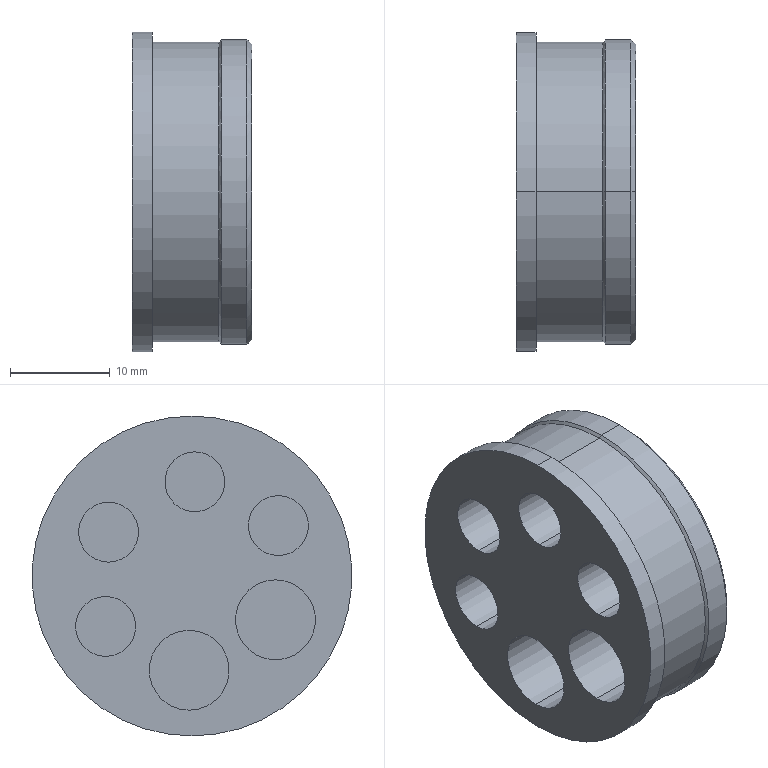Part | SolidWorks | features BaseBody 1 | 1 solid | 34 faces | box 12 x 32 x 32 mm | volume 5499 mm3 | cylinder 20 | plane 10 | cone 4 | commonest cylinder face diameters 6 x8 8 x4 10 x2 30 x2 30.5 x2 32 x2
STEP:
#1=CARTESIAN_POINT('',(-294.521,1906.544,-93.));
#2=VERTEX_POINT('',#1);
#3=CARTESIAN_POINT('',(-294.521,1906.544,-103.));
#4=VERTEX_POINT('',#3);
#5=CARTESIAN_POINT('',(-294.521,1906.544,-98.));
#6=DIRECTION('',(1.,0.,0.));
#7=DIRECTION('',(0.,0.,-1.));
#8=AXIS2_PLACEMENT_3D('',#5,#6,#7);
#9=CIRCLE('',#8,5.);
#10=EDGE_CURVE('',#2,#4,#9,.T.);
#11=ORIENTED_EDGE('',*,*,#10,.F.);
#12=CARTESIAN_POINT('',(-284.521,1906.544,-93.));
#13=VERTEX_POINT('',#12);
#14=CARTESIAN_POINT('',(-289.521,1906.544,-93.));
#15=DIRECTION('',(1.,0.,0.));
#16=VECTOR('',#15,1000.);
#17=LINE('',#14,#16);
#18=EDGE_CURVE('',#2,#13,#17,.T.);
#19=ORIENTED_EDGE('',*,*,#18,.T.);
#20=CARTESIAN_POINT('',(-284.521,1906.544,-103.));
#21=VERTEX_POINT('',#20);
#22=CARTESIAN_POINT('',(-284.521,1906.544,-98.));
#23=DIRECTION('',(-1.,0.,0.));
#24=DIRECTION('',(0.,0.,-1.));
#25=AXIS2_PLACEMENT_3D('',#22,#23,#24);
#26=CIRCLE('',#25,5.);
#27=EDGE_CURVE('',#21,#13,#26,.T.);
#28=ORIENTED_EDGE('',*,*,#27,.F.);
#29=CARTESIAN_POINT('',(-289.521,1906.544,-103.));
#30=DIRECTION('',(1.,0.,0.));
#31=VECTOR('',#30,1000.);
#32=LINE('',#29,#31);
#33=EDGE_CURVE('',#4,#21,#32,.T.);
#34=ORIENTED_EDGE('',*,*,#33,.F.);
#35=EDGE_LOOP('',(#11,#19,#28,#34));
#36=FACE_OUTER_BOUND('',#35,.T.);
#37=CARTESIAN_POINT('',(-289.521,1906.544,-98.));
#38=DIRECTION('',(1.,0.,0.));
#39=DIRECTION('',(0.,0.,-1.));
#40=AXIS2_PLACEMENT_3D('',#37,#38,#39);
#41=CYLINDRICAL_SURFACE('',#40,5.);
#42=ADVANCED_FACE('',(#36),#41,.F.);
#43=CARTESIAN_POINT('',(-284.521,1906.544,-112.75));
#44=VERTEX_POINT('',#43);
#45=CARTESIAN_POINT('',(-284.521,1906.544,-83.25));
#46=VERTEX_POINT('',#45);
#47=CARTESIAN_POINT('',(-284.521,1906.544,-98.));
#48=DIRECTION('',(1.,0.,0.));
#49=DIRECTION('',(0.,0.,1.));
#50=AXIS2_PLACEMENT_3D('',#47,#48,#49);
#51=CIRCLE('',#50,14.75);
#52=EDGE_CURVE('',#44,#46,#51,.T.);
#53=ORIENTED_EDGE('',*,*,#52,.F.);
#54=CARTESIAN_POINT('',(-285.021,1906.544,-113.25));
#55=VERTEX_POINT('',#54);
#56=CARTESIAN_POINT('',(-285.021,1906.544,-113.25));
#57=DIRECTION('',(-0.7071,0.,-0.7071));
#58=VECTOR('',#57,1000.);
#59=LINE('',#56,#58);
#60=EDGE_CURVE('',#44,#55,#59,.T.);
#61=ORIENTED_EDGE('',*,*,#60,.T.);
#62=CARTESIAN_POINT('',(-285.021,1906.544,-82.75));
#63=VERTEX_POINT('',#62);
#64=CARTESIAN_POINT('',(-285.021,1906.544,-98.));
#65=DIRECTION('',(1.,0.,0.));
#66=DIRECTION('',(0.,-0.5043,-0.8635));
#67=AXIS2_PLACEMENT_3D('',#64,#65,#66);
#68=CIRCLE('',#67,15.25);
#69=EDGE_CURVE('',#55,#63,#68,.T.);
#70=ORIENTED_EDGE('',*,*,#69,.T.);
#71=CARTESIAN_POINT('',(-285.021,1906.544,-82.75));
#72=DIRECTION('',(-0.7071,0.,0.7071));
#73=VECTOR('',#72,1000.);
#74=LINE('',#71,#73);
#75=EDGE_CURVE('',#46,#63,#74,.T.);
#76=ORIENTED_EDGE('',*,*,#75,.F.);
#77=EDGE_LOOP('',(#53,#61,#70,#76));
#78=FACE_OUTER_BOUND('',#77,.T.);
#79=CARTESIAN_POINT('',(-285.021,1906.544,-98.));
#80=DIRECTION('',(-1.,0.,0.));
#81=DIRECTION('',(0.,0.,1.));
#82=AXIS2_PLACEMENT_3D('',#79,#80,#81);
#83=CONICAL_SURFACE('',#82,15.25,0.7854);
#84=ADVANCED_FACE('',(#78),#83,.T.);
#85=ORIENTED_EDGE('',*,*,#69,.F.);
#86=CARTESIAN_POINT('',(-287.571,1906.544,-113.25));
#87=VERTEX_POINT('',#86);
#88=CARTESIAN_POINT('',(-284.521,1906.544,-113.25));
#89=DIRECTION('',(-1.,0.,0.));
#90=VECTOR('',#89,1000.);
#91=LINE('',#88,#90);
#92=EDGE_CURVE('',#55,#87,#91,.T.);
#93=ORIENTED_EDGE('',*,*,#92,.T.);
#94=CARTESIAN_POINT('',(-287.571,1906.544,-82.75));
#95=VERTEX_POINT('',#94);
#96=CARTESIAN_POINT('',(-287.571,1906.544,-98.));
#97=DIRECTION('',(1.,0.,0.));
#98=DIRECTION('',(0.,0.,1.));
#99=AXIS2_PLACEMENT_3D('',#96,#97,#98);
#100=CIRCLE('',#99,15.25);
#101=EDGE_CURVE('',#87,#95,#100,.T.);
#102=ORIENTED_EDGE('',*,*,#101,.T.);
#103=CARTESIAN_POINT('',(-284.521,1906.544,-82.75));
#104=DIRECTION('',(-1.,0.,0.));
#105=VECTOR('',#104,1000.);
#106=LINE('',#103,#105);
#107=EDGE_CURVE('',#63,#95,#106,.T.);
#108=ORIENTED_EDGE('',*,*,#107,.F.);
#109=EDGE_LOOP('',(#85,#93,#102,#108));
#110=FACE_OUTER_BOUND('',#109,.T.);
#111=CARTESIAN_POINT('',(-284.521,1906.544,-98.));
#112=DIRECTION('',(-1.,0.,0.));
#113=DIRECTION('',(0.,0.,1.));
#114=AXIS2_PLACEMENT_3D('',#111,#112,#113);
#115=CYLINDRICAL_SURFACE('',#114,15.25);
#116=ADVANCED_FACE('',(#110),#115,.T.);
#117=CARTESIAN_POINT('',(-287.821,1906.544,-113.));
#118=VERTEX_POINT('',#117);
#119=CARTESIAN_POINT('',(-287.821,1906.544,-83.));
#120=VERTEX_POINT('',#119);
#121=CARTESIAN_POINT('',(-287.821,1906.544,-98.));
#122=DIRECTION('',(1.,0.,0.));
#123=DIRECTION('',(0.,0.5043,0.8635));
#124=AXIS2_PLACEMENT_3D('',#121,#122,#123);
#125=CIRCLE('',#124,15.);
#126=EDGE_CURVE('',#118,#120,#125,.T.);
#127=ORIENTED_EDGE('',*,*,#126,.T.);
#128=CARTESIAN_POINT('',(-287.571,1906.544,-82.75));
#129=DIRECTION('',(0.7071,0.,0.7071));
#130=VECTOR('',#129,1000.);
#131=LINE('',#128,#130);
#132=EDGE_CURVE('',#120,#95,#131,.T.);
#133=ORIENTED_EDGE('',*,*,#132,.T.);
#134=ORIENTED_EDGE('',*,*,#101,.F.);
#135=CARTESIAN_POINT('',(-287.571,1906.544,-113.25));
#136=DIRECTION('',(0.7071,0.,-0.7071));
#137=VECTOR('',#136,1000.);
#138=LINE('',#135,#137);
#139=EDGE_CURVE('',#118,#87,#138,.T.);
#140=ORIENTED_EDGE('',*,*,#139,.F.);
#141=EDGE_LOOP('',(#127,#133,#134,#140));
#142=FACE_OUTER_BOUND('',#141,.T.);
#143=CARTESIAN_POINT('',(-287.571,1906.544,-98.));
#144=DIRECTION('',(1.,0.,0.));
#145=DIRECTION('',(0.,0.,-1.));
#146=AXIS2_PLACEMENT_3D('',#143,#144,#145);
#147=CONICAL_SURFACE('',#146,15.25,0.7854);
#148=ADVANCED_FACE('',(#142),#147,.T.);
#149=ORIENTED_EDGE('',*,*,#126,.F.);
#150=CARTESIAN_POINT('',(-294.521,1906.544,-113.));
#151=VERTEX_POINT('',#150);
#152=CARTESIAN_POINT('',(-284.521,1906.544,-113.));
#153=DIRECTION('',(-1.,0.,0.));
#154=VECTOR('',#153,1000.);
#155=LINE('',#152,#154);
#156=EDGE_CURVE('',#118,#151,#155,.T.);
#157=ORIENTED_EDGE('',*,*,#156,.T.);
#158=CARTESIAN_POINT('',(-294.521,1906.544,-83.));
#159=VERTEX_POINT('',#158);
#160=CARTESIAN_POINT('',(-294.521,1906.544,-98.));
#161=DIRECTION('',(1.,0.,0.));
#162=DIRECTION('',(0.,0.,1.));
#163=AXIS2_PLACEMENT_3D('',#160,#161,#162);
#164=CIRCLE('',#163,15.);
#165=EDGE_CURVE('',#151,#159,#164,.T.);
#166=ORIENTED_EDGE('',*,*,#165,.T.);
#167=CARTESIAN_POINT('',(-284.521,1906.544,-83.));
#168=DIRECTION('',(-1.,0.,0.));
#169=VECTOR('',#168,1000.);
#170=LINE('',#167,#169);
#171=EDGE_CURVE('',#120,#159,#170,.T.);
#172=ORIENTED_EDGE('',*,*,#171,.F.);
#173=EDGE_LOOP('',(#149,#157,#166,#172));
#174=FACE_OUTER_BOUND('',#173,.T.);
#175=CARTESIAN_POINT('',(-284.521,1906.544,-98.));
#176=DIRECTION('',(-1.,0.,0.));
#177=DIRECTION('',(0.,0.,1.));
#178=AXIS2_PLACEMENT_3D('',#175,#176,#177);
#179=CYLINDRICAL_SURFACE('',#178,15.);
#180=ADVANCED_FACE('',(#174),#179,.T.);
#181=CARTESIAN_POINT('',(-294.521,1906.544,-114.));
#182=VERTEX_POINT('',#181);
#183=CARTESIAN_POINT('',(-294.521,1906.544,-82.));
#184=VERTEX_POINT('',#183);
#185=CARTESIAN_POINT('',(-294.521,1906.544,-98.));
#186=DIRECTION('',(1.,0.,0.));
#187=DIRECTION('',(0.,0.,1.));
#188=AXIS2_PLACEMENT_3D('',#185,#186,#187);
#189=CIRCLE('',#188,16.);
#190=EDGE_CURVE('',#182,#184,#189,.T.);
#191=ORIENTED_EDGE('',*,*,#190,.F.);
#192=CARTESIAN_POINT('',(-296.521,1906.544,-114.));
#193=VERTEX_POINT('',#192);
#194=CARTESIAN_POINT('',(-294.521,1906.544,-114.));
#195=DIRECTION('',(-1.,0.,0.));
#196=VECTOR('',#195,1000.);
#197=LINE('',#194,#196);
#198=EDGE_CURVE('',#182,#193,#197,.T.);
#199=ORIENTED_EDGE('',*,*,#198,.T.);
#200=CARTESIAN_POINT('',(-296.521,1906.544,-82.));
#201=VERTEX_POINT('',#200);
#202=CARTESIAN_POINT('',(-296.521,1906.544,-98.));
#203=DIRECTION('',(1.,0.,0.));
#204=DIRECTION('',(0.,0.,1.));
#205=AXIS2_PLACEMENT_3D('',#202,#203,#204);
#206=CIRCLE('',#205,16.);
#207=EDGE_CURVE('',#193,#201,#206,.T.);
#208=ORIENTED_EDGE('',*,*,#207,.T.);
#209=CARTESIAN_POINT('',(-294.521,1906.544,-82.));
#210=DIRECTION('',(-1.,0.,0.));
#211=VECTOR('',#210,1000.);
#212=LINE('',#209,#211);
#213=EDGE_CURVE('',#184,#201,#212,.T.);
#214=ORIENTED_EDGE('',*,*,#213,.F.);
#215=EDGE_LOOP('',(#191,#199,#208,#214));
#216=FACE_OUTER_BOUND('',#215,.T.);
#217=CARTESIAN_POINT('',(-294.521,1906.544,-98.));
#218=DIRECTION('',(-1.,0.,0.));
#219=DIRECTION('',(0.,0.,1.));
#220=AXIS2_PLACEMENT_3D('',#217,#218,#219);
#221=CYLINDRICAL_SURFACE('',#220,16.);
#222=ADVANCED_FACE('',(#216),#221,.T.);
#223=CARTESIAN_POINT('',(-285.021,1906.827,-111.43));
#224=VERTEX_POINT('',#223);
#225=CARTESIAN_POINT('',(-285.021,1906.827,-103.43));
#226=VERTEX_POINT('',#225);
#227=CARTESIAN_POINT('',(-285.021,1906.827,-107.43));
#228=DIRECTION('',(-1.,0.,0.));
#229=DIRECTION('',(0.,0.,1.));
#230=AXIS2_PLACEMENT_3D('',#227,#228,#229);
#231=CIRCLE('',#230,4.);
#232=EDGE_CURVE('',#224,#226,#231,.T.);
#233=ORIENTED_EDGE('',*,*,#232,.F.);
#234=CARTESIAN_POINT('',(-296.521,1906.827,-111.43));
#235=VERTEX_POINT('',#234);
#236=CARTESIAN_POINT('',(-290.771,1906.827,-111.43));
#237=DIRECTION('',(-1.,0.,0.));
#238=VECTOR('',#237,1000.);
#239=LINE('',#236,#238);
#240=EDGE_CURVE('',#224,#235,#239,.T.);
#241=ORIENTED_EDGE('',*,*,#240,.T.);
#242=CARTESIAN_POINT('',(-296.521,1906.827,-103.43));
#243=VERTEX_POINT('',#242);
#244=CARTESIAN_POINT('',(-296.521,1906.827,-107.43));
#245=DIRECTION('',(-1.,0.,0.));
#246=DIRECTION('',(0.,0.,1.));
#247=AXIS2_PLACEMENT_3D('',#244,#245,#246);
#248=CIRCLE('',#247,4.);
#249=EDGE_CURVE('',#235,#243,#248,.T.);
#250=ORIENTED_EDGE('',*,*,#249,.T.);
#251=CARTESIAN_POINT('',(-290.771,1906.827,-103.43));
#252=DIRECTION('',(-1.,0.,0.));
#253=VECTOR('',#252,1000.);
#254=LINE('',#251,#253);
#255=EDGE_CURVE('',#226,#243,#254,.T.);
#256=ORIENTED_EDGE('',*,*,#255,.F.);
#257=EDGE_LOOP('',(#233,#241,#250,#256));
#258=FACE_OUTER_BOUND('',#257,.T.);
#259=CARTESIAN_POINT('',(-290.771,1906.827,-107.43));
#260=DIRECTION('',(-1.,0.,0.));
#261=DIRECTION('',(0.,0.,1.));
#262=AXIS2_PLACEMENT_3D('',#259,#260,#261);
#263=CYLINDRICAL_SURFACE('',#262,4.);
#264=ADVANCED_FACE('',(#258),#263,.F.);
#265=CARTESIAN_POINT('',(-285.021,1906.261,-91.57));
#266=VERTEX_POINT('',#265);
#267=CARTESIAN_POINT('',(-285.021,1906.261,-85.57));
#268=VERTEX_POINT('',#267);
#269=CARTESIAN_POINT('',(-285.021,1906.261,-88.57));
#270=DIRECTION('',(-1.,0.,0.));
#271=DIRECTION('',(0.,0.,1.));
#272=AXIS2_PLACEMENT_3D('',#269,#270,#271);
#273=CIRCLE('',#272,3.);
#274=EDGE_CURVE('',#266,#268,#273,.T.);
#275=ORIENTED_EDGE('',*,*,#274,.F.);
#276=CARTESIAN_POINT('',(-296.521,1906.261,-91.57));
#277=VERTEX_POINT('',#276);
#278=CARTESIAN_POINT('',(-290.771,1906.261,-91.57));
#279=DIRECTION('',(-1.,0.,0.));
#280=VECTOR('',#279,1000.);
#281=LINE('',#278,#280);
#282=EDGE_CURVE('',#266,#277,#281,.T.);
#283=ORIENTED_EDGE('',*,*,#282,.T.);
#284=CARTESIAN_POINT('',(-296.521,1906.261,-85.57));
#285=VERTEX_POINT('',#284);
#286=CARTESIAN_POINT('',(-296.521,1906.261,-88.57));
#287=DIRECTION('',(-1.,0.,0.));
#288=DIRECTION('',(0.,0.,1.));
#289=AXIS2_PLACEMENT_3D('',#286,#287,#288);
#290=CIRCLE('',#289,3.);
#291=EDGE_CURVE('',#277,#285,#290,.T.);
#292=ORIENTED_EDGE('',*,*,#291,.T.);
#293=CARTESIAN_POINT('',(-290.771,1906.261,-85.57));
#294=DIRECTION('',(-1.,0.,0.));
#295=VECTOR('',#294,1000.);
#296=LINE('',#293,#295);
#297=EDGE_CURVE('',#268,#285,#296,.T.);
#298=ORIENTED_EDGE('',*,*,#297,.F.);
#299=EDGE_LOOP('',(#275,#283,#292,#298));
#300=FACE_OUTER_BOUND('',#299,.T.);
#301=CARTESIAN_POINT('',(-290.771,1906.261,-88.57));
#302=DIRECTION('',(-1.,0.,0.));
#303=DIRECTION('',(0.,0.,1.));
#304=AXIS2_PLACEMENT_3D('',#301,#302,#303);
#305=CYLINDRICAL_SURFACE('',#304,3.);
#306=ADVANCED_FACE('',(#300),#305,.F.);
#307=CARTESIAN_POINT('',(-285.021,1915.179,-106.043));
#308=VERTEX_POINT('',#307);
#309=CARTESIAN_POINT('',(-285.021,1915.179,-100.043));
#310=VERTEX_POINT('',#309);
#311=CARTESIAN_POINT('',(-285.021,1915.179,-103.043));
#312=DIRECTION('',(-1.,0.,0.));
#313=DIRECTION('',(0.,0.,1.));
#314=AXIS2_PLACEMENT_3D('',#311,#312,#313);
#315=CIRCLE('',#314,3.);
#316=EDGE_CURVE('',#308,#310,#315,.T.);
#317=ORIENTED_EDGE('',*,*,#316,.F.);
#318=CARTESIAN_POINT('',(-296.521,1915.179,-106.043));
#319=VERTEX_POINT('',#318);
#320=CARTESIAN_POINT('',(-290.771,1915.179,-106.043));
#321=DIRECTION('',(-1.,0.,0.));
#322=VECTOR('',#321,1000.);
#323=LINE('',#320,#322);
#324=EDGE_CURVE('',#308,#319,#323,.T.);
#325=ORIENTED_EDGE('',*,*,#324,.T.);
#326=CARTESIAN_POINT('',(-296.521,1915.179,-100.043));
#327=VERTEX_POINT('',#326);
#328=CARTESIAN_POINT('',(-296.521,1915.179,-103.043));
#329=DIRECTION('',(-1.,0.,0.));
#330=DIRECTION('',(0.,0.,1.));
#331=AXIS2_PLACEMENT_3D('',#328,#329,#330);
#332=CIRCLE('',#331,3.);
#333=EDGE_CURVE('',#319,#327,#332,.T.);
#334=ORIENTED_EDGE('',*,*,#333,.T.);
#335=CARTESIAN_POINT('',(-290.771,1915.179,-100.043));
#336=DIRECTION('',(-1.,0.,0.));
#337=VECTOR('',#336,1000.);
#338=LINE('',#335,#337);
#339=EDGE_CURVE('',#310,#327,#338,.T.);
#340=ORIENTED_EDGE('',*,*,#339,.F.);
#341=EDGE_LOOP('',(#317,#325,#334,#340));
#342=FACE_OUTER_BOUND('',#341,.T.);
#343=CARTESIAN_POINT('',(-290.771,1915.179,-103.043));
#344=DIRECTION('',(-1.,0.,0.));
#345=DIRECTION('',(0.,0.,1.));
#346=AXIS2_PLACEMENT_3D('',#343,#344,#345);
#347=CYLINDRICAL_SURFACE('',#346,3.);
#348=ADVANCED_FACE('',(#342),#347,.F.);
#349=CARTESIAN_POINT('',(-285.021,1897.909,-95.957));
#350=VERTEX_POINT('',#349);
#351=CARTESIAN_POINT('',(-285.021,1897.909,-89.957));
#352=VERTEX_POINT('',#351);
#353=CARTESIAN_POINT('',(-285.021,1897.909,-92.957));
#354=DIRECTION('',(-1.,0.,0.));
#355=DIRECTION('',(0.,0.,1.));
#356=AXIS2_PLACEMENT_3D('',#353,#354,#355);
#357=CIRCLE('',#356,3.);
#358=EDGE_CURVE('',#350,#352,#357,.T.);
#359=ORIENTED_EDGE('',*,*,#358,.F.);
#360=CARTESIAN_POINT('',(-296.521,1897.909,-95.957));
#361=VERTEX_POINT('',#360);
#362=CARTESIAN_POINT('',(-290.771,1897.909,-95.957));
#363=DIRECTION('',(-1.,0.,0.));
#364=VECTOR('',#363,1000.);
#365=LINE('',#362,#364);
#366=EDGE_CURVE('',#350,#361,#365,.T.);
#367=ORIENTED_EDGE('',*,*,#366,.T.);
#368=CARTESIAN_POINT('',(-296.521,1897.909,-89.957));
#369=VERTEX_POINT('',#368);
#370=CARTESIAN_POINT('',(-296.521,1897.909,-92.957));
#371=DIRECTION('',(-1.,0.,0.));
#372=DIRECTION('',(0.,0.,1.));
#373=AXIS2_PLACEMENT_3D('',#370,#371,#372);
#374=CIRCLE('',#373,3.);
#375=EDGE_CURVE('',#361,#369,#374,.T.);
#376=ORIENTED_EDGE('',*,*,#375,.T.);
#377=CARTESIAN_POINT('',(-290.771,1897.909,-89.957));
#378=DIRECTION('',(-1.,0.,0.));
#379=VECTOR('',#378,1000.);
#380=LINE('',#377,#379);
#381=EDGE_CURVE('',#352,#369,#380,.T.);
#382=ORIENTED_EDGE('',*,*,#381,.F.);
#383=EDGE_LOOP('',(#359,#367,#376,#382));
#384=FACE_OUTER_BOUND('',#383,.T.);
#385=CARTESIAN_POINT('',(-290.771,1897.909,-92.957));
#386=DIRECTION('',(-1.,0.,0.));
#387=DIRECTION('',(0.,0.,1.));
#388=AXIS2_PLACEMENT_3D('',#385,#386,#387);
#389=CYLINDRICAL_SURFACE('',#388,3.);
#390=ADVANCED_FACE('',(#384),#389,.F.);
#391=CARTESIAN_POINT('',(-285.021,1914.896,-96.613));
#392=VERTEX_POINT('',#391);
#393=CARTESIAN_POINT('',(-285.021,1914.896,-90.613));
#394=VERTEX_POINT('',#393);
#395=CARTESIAN_POINT('',(-285.021,1914.896,-93.613));
#396=DIRECTION('',(-1.,0.,0.));
#397=DIRECTION('',(0.,0.,1.));
#398=AXIS2_PLACEMENT_3D('',#395,#396,#397);
#399=CIRCLE('',#398,3.);
#400=EDGE_CURVE('',#392,#394,#399,.T.);
#401=ORIENTED_EDGE('',*,*,#400,.F.);
#402=CARTESIAN_POINT('',(-296.521,1914.896,-96.613));
#403=VERTEX_POINT('',#402);
#404=CARTESIAN_POINT('',(-290.771,1914.896,-96.613));
#405=DIRECTION('',(-1.,0.,0.));
#406=VECTOR('',#405,1000.);
#407=LINE('',#404,#406);
#408=EDGE_CURVE('',#392,#403,#407,.T.);
#409=ORIENTED_EDGE('',*,*,#408,.T.);
#410=CARTESIAN_POINT('',(-296.521,1914.896,-90.613));
#411=VERTEX_POINT('',#410);
#412=CARTESIAN_POINT('',(-296.521,1914.896,-93.613));
#413=DIRECTION('',(-1.,0.,0.));
#414=DIRECTION('',(0.,0.,1.));
#415=AXIS2_PLACEMENT_3D('',#412,#413,#414);
#416=CIRCLE('',#415,3.);
#417=EDGE_CURVE('',#403,#411,#416,.T.);
#418=ORIENTED_EDGE('',*,*,#417,.T.);
#419=CARTESIAN_POINT('',(-290.771,1914.896,-90.613));
#420=DIRECTION('',(-1.,0.,0.));
#421=VECTOR('',#420,1000.);
#422=LINE('',#419,#421);
#423=EDGE_CURVE('',#394,#411,#422,.T.);
#424=ORIENTED_EDGE('',*,*,#423,.F.);
#425=EDGE_LOOP('',(#401,#409,#418,#424));
#426=FACE_OUTER_BOUND('',#425,.T.);
#427=CARTESIAN_POINT('',(-290.771,1914.896,-93.613));
#428=DIRECTION('',(-1.,0.,0.));
#429=DIRECTION('',(0.,0.,1.));
#430=AXIS2_PLACEMENT_3D('',#427,#428,#429);
#431=CYLINDRICAL_SURFACE('',#430,3.);
#432=ADVANCED_FACE('',(#426),#431,.F.);
#433=CARTESIAN_POINT('',(-285.021,1898.192,-106.387));
#434=VERTEX_POINT('',#433);
#435=CARTESIAN_POINT('',(-285.021,1898.192,-98.387));
#436=VERTEX_POINT('',#435);
#437=CARTESIAN_POINT('',(-285.021,1898.192,-102.387));
#438=DIRECTION('',(-1.,0.,0.));
#439=DIRECTION('',(0.,0.,1.));
#440=AXIS2_PLACEMENT_3D('',#437,#438,#439);
#441=CIRCLE('',#440,4.);
#442=EDGE_CURVE('',#434,#436,#441,.T.);
#443=ORIENTED_EDGE('',*,*,#442,.F.);
#444=CARTESIAN_POINT('',(-296.521,1898.192,-106.387));
#445=VERTEX_POINT('',#444);
#446=CARTESIAN_POINT('',(-290.771,1898.192,-106.387));
#447=DIRECTION('',(-1.,0.,0.));
#448=VECTOR('',#447,1000.);
#449=LINE('',#446,#448);
#450=EDGE_CURVE('',#434,#445,#449,.T.);
#451=ORIENTED_EDGE('',*,*,#450,.T.);
#452=CARTESIAN_POINT('',(-296.521,1898.192,-98.387));
#453=VERTEX_POINT('',#452);
#454=CARTESIAN_POINT('',(-296.521,1898.192,-102.387));
#455=DIRECTION('',(-1.,0.,0.));
#456=DIRECTION('',(0.,0.,1.));
#457=AXIS2_PLACEMENT_3D('',#454,#455,#456);
#458=CIRCLE('',#457,4.);
#459=EDGE_CURVE('',#445,#453,#458,.T.);
#460=ORIENTED_EDGE('',*,*,#459,.T.);
#461=CARTESIAN_POINT('',(-290.771,1898.192,-98.387));
#462=DIRECTION('',(-1.,0.,0.));
#463=VECTOR('',#462,1000.);
#464=LINE('',#461,#463);
#465=EDGE_CURVE('',#436,#453,#464,.T.);
#466=ORIENTED_EDGE('',*,*,#465,.F.);
#467=EDGE_LOOP('',(#443,#451,#460,#466));
#468=FACE_OUTER_BOUND('',#467,.T.);
#469=CARTESIAN_POINT('',(-290.771,1898.192,-102.387));
#470=DIRECTION('',(-1.,0.,0.));
#471=DIRECTION('',(0.,0.,1.));
#472=AXIS2_PLACEMENT_3D('',#469,#470,#471);
#473=CYLINDRICAL_SURFACE('',#472,4.);
#474=ADVANCED_FACE('',(#468),#473,.F.);
#475=ORIENTED_EDGE('',*,*,#27,.T.);
#476=CARTESIAN_POINT('',(-284.521,1906.544,-98.));
#477=DIRECTION('',(-1.,0.,0.));
#478=DIRECTION('',(0.,0.,-1.));
#479=AXIS2_PLACEMENT_3D('',#476,#477,#478);
#480=CIRCLE('',#479,5.);
#481=EDGE_CURVE('',#13,#21,#480,.T.);
#482=ORIENTED_EDGE('',*,*,#481,.T.);
#483=EDGE_LOOP('',(#475,#482));
#484=FACE_BOUND('',#483,.T.);
#485=CARTESIAN_POINT('',(-284.521,1906.544,-98.));
#486=DIRECTION('',(1.,0.,0.));
#487=DIRECTION('',(0.,0.,1.));
#488=AXIS2_PLACEMENT_3D('',#485,#486,#487);
#489=CIRCLE('',#488,14.75);
#490=EDGE_CURVE('',#46,#44,#489,.T.);
#491=ORIENTED_EDGE('',*,*,#490,.T.);
#492=ORIENTED_EDGE('',*,*,#52,.T.);
#493=EDGE_LOOP('',(#491,#492));
#494=FACE_OUTER_BOUND('',#493,.T.);
#495=CARTESIAN_POINT('',(-284.521,1906.544,-98.));
#496=DIRECTION('',(1.,0.,0.));
#497=DIRECTION('',(0.,0.,-1.));
#498=AXIS2_PLACEMENT_3D('',#495,#496,#497);
#499=PLANE('',#498);
#500=ADVANCED_FACE('',(#484,#494),#499,.T.);
#501=ORIENTED_EDGE('',*,*,#18,.F.);
#502=CARTESIAN_POINT('',(-294.521,1906.544,-98.));
#503=DIRECTION('',(1.,0.,0.));
#504=DIRECTION('',(0.,0.,-1.));
#505=AXIS2_PLACEMENT_3D('',#502,#503,#504);
#506=CIRCLE('',#505,5.);
#507=EDGE_CURVE('',#4,#2,#506,.T.);
#508=ORIENTED_EDGE('',*,*,#507,.F.);
#509=ORIENTED_EDGE('',*,*,#33,.T.);
#510=ORIENTED_EDGE('',*,*,#481,.F.);
#511=EDGE_LOOP('',(#501,#508,#509,#510));
#512=FACE_OUTER_BOUND('',#511,.T.);
#513=CARTESIAN_POINT('',(-289.521,1906.544,-98.));
#514=DIRECTION('',(1.,0.,0.));
#515=DIRECTION('',(0.,0.,-1.));
#516=AXIS2_PLACEMENT_3D('',#513,#514,#515);
#517=CYLINDRICAL_SURFACE('',#516,5.);
#518=ADVANCED_FACE('',(#512),#517,.F.);
#519=ORIENTED_EDGE('',*,*,#60,.F.);
#520=ORIENTED_EDGE('',*,*,#490,.F.);
#521=ORIENTED_EDGE('',*,*,#75,.T.);
#522=CARTESIAN_POINT('',(-285.021,1906.544,-98.));
#523=DIRECTION('',(1.,0.,0.));
#524=DIRECTION('',(0.,-0.5043,-0.8635));
#525=AXIS2_PLACEMENT_3D('',#522,#523,#524);
#526=CIRCLE('',#525,15.25);
#527=EDGE_CURVE('',#63,#55,#526,.T.);
#528=ORIENTED_EDGE('',*,*,#527,.T.);
#529=EDGE_LOOP('',(#519,#520,#521,#528));
#530=FACE_OUTER_BOUND('',#529,.T.);
#531=CARTESIAN_POINT('',(-285.021,1906.544,-98.));
#532=DIRECTION('',(-1.,0.,0.));
#533=DIRECTION('',(0.,0.,1.));
#534=AXIS2_PLACEMENT_3D('',#531,#532,#533);
#535=CONICAL_SURFACE('',#534,15.25,0.7854);
#536=ADVANCED_FACE('',(#530),#535,.T.);
#537=ORIENTED_EDGE('',*,*,#507,.T.);
#538=ORIENTED_EDGE('',*,*,#10,.T.);
#539=EDGE_LOOP('',(#537,#538));
#540=FACE_OUTER_BOUND('',#539,.T.);
#541=CARTESIAN_POINT('',(-294.521,1906.544,-98.));
#542=DIRECTION('',(1.,0.,0.));
#543=DIRECTION('',(0.,0.,-1.));
#544=AXIS2_PLACEMENT_3D('',#541,#542,#543);
#545=PLANE('',#544);
#546=ADVANCED_FACE('',(#540),#545,.T.);
#547=ORIENTED_EDGE('',*,*,#92,.F.);
#548=ORIENTED_EDGE('',*,*,#527,.F.);
#549=ORIENTED_EDGE('',*,*,#107,.T.);
#550=CARTESIAN_POINT('',(-287.571,1906.544,-98.));
#551=DIRECTION('',(1.,0.,0.));
#552=DIRECTION('',(0.,0.,1.));
#553=AXIS2_PLACEMENT_3D('',#550,#551,#552);
#554=CIRCLE('',#553,15.25);
#555=EDGE_CURVE('',#95,#87,#554,.T.);
#556=ORIENTED_EDGE('',*,*,#555,.T.);
#557=EDGE_LOOP('',(#547,#548,#549,#556));
#558=FACE_OUTER_BOUND('',#557,.T.);
#559=CARTESIAN_POINT('',(-284.521,1906.544,-98.));
#560=DIRECTION('',(-1.,0.,0.));
#561=DIRECTION('',(0.,0.,1.));
#562=AXIS2_PLACEMENT_3D('',#559,#560,#561);
#563=CYLINDRICAL_SURFACE('',#562,15.25);
#564=ADVANCED_FACE('',(#558),#563,.T.);
#565=ORIENTED_EDGE('',*,*,#132,.F.);
#566=CARTESIAN_POINT('',(-287.821,1906.544,-98.));
#567=DIRECTION('',(1.,0.,0.));
#568=DIRECTION('',(0.,0.5043,0.8635));
#569=AXIS2_PLACEMENT_3D('',#566,#567,#568);
#570=CIRCLE('',#569,15.);
#571=EDGE_CURVE('',#120,#118,#570,.T.);
#572=ORIENTED_EDGE('',*,*,#571,.T.);
#573=ORIENTED_EDGE('',*,*,#139,.T.);
#574=ORIENTED_EDGE('',*,*,#555,.F.);
#575=EDGE_LOOP('',(#565,#572,#573,#574));
#576=FACE_OUTER_BOUND('',#575,.T.);
#577=CARTESIAN_POINT('',(-287.571,1906.544,-98.));
#578=DIRECTION('',(1.,0.,0.));
#579=DIRECTION('',(0.,0.,-1.));
#580=AXIS2_PLACEMENT_3D('',#577,#578,#579);
#581=CONICAL_SURFACE('',#580,15.25,0.7854);
#582=ADVANCED_FACE('',(#576),#581,.T.);
#583=ORIENTED_EDGE('',*,*,#156,.F.);
#584=ORIENTED_EDGE('',*,*,#571,.F.);
#585=ORIENTED_EDGE('',*,*,#171,.T.);
#586=CARTESIAN_POINT('',(-294.521,1906.544,-98.));
#587=DIRECTION('',(1.,0.,0.));
#588=DIRECTION('',(0.,0.,1.));
#589=AXIS2_PLACEMENT_3D('',#586,#587,#588);
#590=CIRCLE('',#589,15.);
#591=EDGE_CURVE('',#159,#151,#590,.T.);
#592=ORIENTED_EDGE('',*,*,#591,.T.);
#593=EDGE_LOOP('',(#583,#584,#585,#592));
#594=FACE_OUTER_BOUND('',#593,.T.);
#595=CARTESIAN_POINT('',(-284.521,1906.544,-98.));
#596=DIRECTION('',(-1.,0.,0.));
#597=DIRECTION('',(0.,0.,1.));
#598=AXIS2_PLACEMENT_3D('',#595,#596,#597);
#599=CYLINDRICAL_SURFACE('',#598,15.);
#600=ADVANCED_FACE('',(#594),#599,.T.);
#601=ORIENTED_EDGE('',*,*,#591,.F.);
#602=ORIENTED_EDGE('',*,*,#165,.F.);
#603=EDGE_LOOP('',(#601,#602));
#604=FACE_BOUND('',#603,.T.);
#605=CARTESIAN_POINT('',(-294.521,1906.544,-98.));
#606=DIRECTION('',(1.,0.,0.));
#607=DIRECTION('',(0.,0.,1.));
#608=AXIS2_PLACEMENT_3D('',#605,#606,#607);
#609=CIRCLE('',#608,16.);
#610=EDGE_CURVE('',#184,#182,#609,.T.);
#611=ORIENTED_EDGE('',*,*,#610,.T.);
#612=ORIENTED_EDGE('',*,*,#190,.T.);
#613=EDGE_LOOP('',(#611,#612));
#614=FACE_OUTER_BOUND('',#613,.T.);
#615=CARTESIAN_POINT('',(-294.521,1906.544,-98.));
#616=DIRECTION('',(1.,0.,0.));
#617=DIRECTION('',(0.,0.,-1.));
#618=AXIS2_PLACEMENT_3D('',#615,#616,#617);
#619=PLANE('',#618);
#620=ADVANCED_FACE('',(#604,#614),#619,.T.);
#621=ORIENTED_EDGE('',*,*,#198,.F.);
#622=ORIENTED_EDGE('',*,*,#610,.F.);
#623=ORIENTED_EDGE('',*,*,#213,.T.);
#624=CARTESIAN_POINT('',(-296.521,1906.544,-98.));
#625=DIRECTION('',(1.,0.,0.));
#626=DIRECTION('',(0.,0.,1.));
#627=AXIS2_PLACEMENT_3D('',#624,#625,#626);
#628=CIRCLE('',#627,16.);
#629=EDGE_CURVE('',#201,#193,#628,.T.);
#630=ORIENTED_EDGE('',*,*,#629,.T.);
#631=EDGE_LOOP('',(#621,#622,#623,#630));
#632=FACE_OUTER_BOUND('',#631,.T.);
#633=CARTESIAN_POINT('',(-294.521,1906.544,-98.));
#634=DIRECTION('',(-1.,0.,0.));
#635=DIRECTION('',(0.,0.,1.));
#636=AXIS2_PLACEMENT_3D('',#633,#634,#635);
#637=CYLINDRICAL_SURFACE('',#636,16.);
#638=ADVANCED_FACE('',(#632),#637,.T.);
#639=CARTESIAN_POINT('',(-296.521,1906.827,-107.43));
#640=DIRECTION('',(-1.,0.,0.));
#641=DIRECTION('',(0.,0.,1.));
#642=AXIS2_PLACEMENT_3D('',#639,#640,#641);
#643=CIRCLE('',#642,4.);
#644=EDGE_CURVE('',#243,#235,#643,.T.);
#645=ORIENTED_EDGE('',*,*,#644,.F.);
#646=ORIENTED_EDGE('',*,*,#249,.F.);
#647=EDGE_LOOP('',(#645,#646));
#648=FACE_BOUND('',#647,.T.);
#649=CARTESIAN_POINT('',(-296.521,1906.261,-88.57));
#650=DIRECTION('',(-1.,0.,0.));
#651=DIRECTION('',(0.,0.,1.));
#652=AXIS2_PLACEMENT_3D('',#649,#650,#651);
#653=CIRCLE('',#652,3.);
#654=EDGE_CURVE('',#285,#277,#653,.T.);
#655=ORIENTED_EDGE('',*,*,#654,.F.);
#656=ORIENTED_EDGE('',*,*,#291,.F.);
#657=EDGE_LOOP('',(#655,#656));
#658=FACE_BOUND('',#657,.T.);
#659=CARTESIAN_POINT('',(-296.521,1915.179,-103.043));
#660=DIRECTION('',(-1.,0.,0.));
#661=DIRECTION('',(0.,0.,1.));
#662=AXIS2_PLACEMENT_3D('',#659,#660,#661);
#663=CIRCLE('',#662,3.);
#664=EDGE_CURVE('',#327,#319,#663,.T.);
#665=ORIENTED_EDGE('',*,*,#664,.F.);
#666=ORIENTED_EDGE('',*,*,#333,.F.);
#667=EDGE_LOOP('',(#665,#666));
#668=FACE_BOUND('',#667,.T.);
#669=CARTESIAN_POINT('',(-296.521,1897.909,-92.957));
#670=DIRECTION('',(-1.,0.,0.));
#671=DIRECTION('',(0.,0.,1.));
#672=AXIS2_PLACEMENT_3D('',#669,#670,#671);
#673=CIRCLE('',#672,3.);
#674=EDGE_CURVE('',#369,#361,#673,.T.);
#675=ORIENTED_EDGE('',*,*,#674,.F.);
#676=ORIENTED_EDGE('',*,*,#375,.F.);
#677=EDGE_LOOP('',(#675,#676));
#678=FACE_BOUND('',#677,.T.);
#679=CARTESIAN_POINT('',(-296.521,1914.896,-93.613));
#680=DIRECTION('',(-1.,0.,0.));
#681=DIRECTION('',(0.,0.,1.));
#682=AXIS2_PLACEMENT_3D('',#679,#680,#681);
#683=CIRCLE('',#682,3.);
#684=EDGE_CURVE('',#411,#403,#683,.T.);
#685=ORIENTED_EDGE('',*,*,#684,.F.);
#686=ORIENTED_EDGE('',*,*,#417,.F.);
#687=EDGE_LOOP('',(#685,#686));
#688=FACE_BOUND('',#687,.T.);
#689=CARTESIAN_POINT('',(-296.521,1898.192,-102.387));
#690=DIRECTION('',(-1.,0.,0.));
#691=DIRECTION('',(0.,0.,1.));
#692=AXIS2_PLACEMENT_3D('',#689,#690,#691);
#693=CIRCLE('',#692,4.);
#694=EDGE_CURVE('',#453,#445,#693,.T.);
#695=ORIENTED_EDGE('',*,*,#694,.F.);
#696=ORIENTED_EDGE('',*,*,#459,.F.);
#697=EDGE_LOOP('',(#695,#696));
#698=FACE_BOUND('',#697,.T.);
#699=ORIENTED_EDGE('',*,*,#629,.F.);
#700=ORIENTED_EDGE('',*,*,#207,.F.);
#701=EDGE_LOOP('',(#699,#700));
#702=FACE_OUTER_BOUND('',#701,.T.);
#703=CARTESIAN_POINT('',(-296.521,1906.544,-98.));
#704=DIRECTION('',(1.,0.,0.));
#705=DIRECTION('',(0.,0.,-1.));
#706=AXIS2_PLACEMENT_3D('',#703,#704,#705);
#707=PLANE('',#706);
#708=ADVANCED_FACE('',(#648,#658,#668,#678,#688,#698,#702),#707,.F.);
#709=ORIENTED_EDGE('',*,*,#240,.F.);
#710=CARTESIAN_POINT('',(-285.021,1906.827,-107.43));
#711=DIRECTION('',(-1.,0.,0.));
#712=DIRECTION('',(0.,0.,1.));
#713=AXIS2_PLACEMENT_3D('',#710,#711,#712);
#714=CIRCLE('',#713,4.);
#715=EDGE_CURVE('',#226,#224,#714,.T.);
#716=ORIENTED_EDGE('',*,*,#715,.F.);
#717=ORIENTED_EDGE('',*,*,#255,.T.);
#718=ORIENTED_EDGE('',*,*,#644,.T.);
#719=EDGE_LOOP('',(#709,#716,#717,#718));
#720=FACE_OUTER_BOUND('',#719,.T.);
#721=CARTESIAN_POINT('',(-290.771,1906.827,-107.43));
#722=DIRECTION('',(-1.,0.,0.));
#723=DIRECTION('',(0.,0.,1.));
#724=AXIS2_PLACEMENT_3D('',#721,#722,#723);
#725=CYLINDRICAL_SURFACE('',#724,4.);
#726=ADVANCED_FACE('',(#720),#725,.F.);
#727=ORIENTED_EDGE('',*,*,#282,.F.);
#728=CARTESIAN_POINT('',(-285.021,1906.261,-88.57));
#729=DIRECTION('',(-1.,0.,0.));
#730=DIRECTION('',(0.,0.,1.));
#731=AXIS2_PLACEMENT_3D('',#728,#729,#730);
#732=CIRCLE('',#731,3.);
#733=EDGE_CURVE('',#268,#266,#732,.T.);
#734=ORIENTED_EDGE('',*,*,#733,.F.);
#735=ORIENTED_EDGE('',*,*,#297,.T.);
#736=ORIENTED_EDGE('',*,*,#654,.T.);
#737=EDGE_LOOP('',(#727,#734,#735,#736));
#738=FACE_OUTER_BOUND('',#737,.T.);
#739=CARTESIAN_POINT('',(-290.771,1906.261,-88.57));
#740=DIRECTION('',(-1.,0.,0.));
#741=DIRECTION('',(0.,0.,1.));
#742=AXIS2_PLACEMENT_3D('',#739,#740,#741);
#743=CYLINDRICAL_SURFACE('',#742,3.);
#744=ADVANCED_FACE('',(#738),#743,.F.);
#745=ORIENTED_EDGE('',*,*,#324,.F.);
#746=CARTESIAN_POINT('',(-285.021,1915.179,-103.043));
#747=DIRECTION('',(-1.,0.,0.));
#748=DIRECTION('',(0.,0.,1.));
#749=AXIS2_PLACEMENT_3D('',#746,#747,#748);
#750=CIRCLE('',#749,3.);
#751=EDGE_CURVE('',#310,#308,#750,.T.);
#752=ORIENTED_EDGE('',*,*,#751,.F.);
#753=ORIENTED_EDGE('',*,*,#339,.T.);
#754=ORIENTED_EDGE('',*,*,#664,.T.);
#755=EDGE_LOOP('',(#745,#752,#753,#754));
#756=FACE_OUTER_BOUND('',#755,.T.);
#757=CARTESIAN_POINT('',(-290.771,1915.179,-103.043));
#758=DIRECTION('',(-1.,0.,0.));
#759=DIRECTION('',(0.,0.,1.));
#760=AXIS2_PLACEMENT_3D('',#757,#758,#759);
#761=CYLINDRICAL_SURFACE('',#760,3.);
#762=ADVANCED_FACE('',(#756),#761,.F.);
#763=ORIENTED_EDGE('',*,*,#366,.F.);
#764=CARTESIAN_POINT('',(-285.021,1897.909,-92.957));
#765=DIRECTION('',(-1.,0.,0.));
#766=DIRECTION('',(0.,0.,1.));
#767=AXIS2_PLACEMENT_3D('',#764,#765,#766);
#768=CIRCLE('',#767,3.);
#769=EDGE_CURVE('',#352,#350,#768,.T.);
#770=ORIENTED_EDGE('',*,*,#769,.F.);
#771=ORIENTED_EDGE('',*,*,#381,.T.);
#772=ORIENTED_EDGE('',*,*,#674,.T.);
#773=EDGE_LOOP('',(#763,#770,#771,#772));
#774=FACE_OUTER_BOUND('',#773,.T.);
#775=CARTESIAN_POINT('',(-290.771,1897.909,-92.957));
#776=DIRECTION('',(-1.,0.,0.));
#777=DIRECTION('',(0.,0.,1.));
#778=AXIS2_PLACEMENT_3D('',#775,#776,#777);
#779=CYLINDRICAL_SURFACE('',#778,3.);
#780=ADVANCED_FACE('',(#774),#779,.F.);
#781=ORIENTED_EDGE('',*,*,#408,.F.);
#782=CARTESIAN_POINT('',(-285.021,1914.896,-93.613));
#783=DIRECTION('',(-1.,0.,0.));
#784=DIRECTION('',(0.,0.,1.));
#785=AXIS2_PLACEMENT_3D('',#782,#783,#784);
#786=CIRCLE('',#785,3.);
#787=EDGE_CURVE('',#394,#392,#786,.T.);
#788=ORIENTED_EDGE('',*,*,#787,.F.);
#789=ORIENTED_EDGE('',*,*,#423,.T.);
#790=ORIENTED_EDGE('',*,*,#684,.T.);
#791=EDGE_LOOP('',(#781,#788,#789,#790));
#792=FACE_OUTER_BOUND('',#791,.T.);
#793=CARTESIAN_POINT('',(-290.771,1914.896,-93.613));
#794=DIRECTION('',(-1.,0.,0.));
#795=DIRECTION('',(0.,0.,1.));
#796=AXIS2_PLACEMENT_3D('',#793,#794,#795);
#797=CYLINDRICAL_SURFACE('',#796,3.);
#798=ADVANCED_FACE('',(#792),#797,.F.);
#799=ORIENTED_EDGE('',*,*,#450,.F.);
#800=CARTESIAN_POINT('',(-285.021,1898.192,-102.387));
#801=DIRECTION('',(-1.,0.,0.));
#802=DIRECTION('',(0.,0.,1.));
#803=AXIS2_PLACEMENT_3D('',#800,#801,#802);
#804=CIRCLE('',#803,4.);
#805=EDGE_CURVE('',#436,#434,#804,.T.);
#806=ORIENTED_EDGE('',*,*,#805,.F.);
#807=ORIENTED_EDGE('',*,*,#465,.T.);
#808=ORIENTED_EDGE('',*,*,#694,.T.);
#809=EDGE_LOOP('',(#799,#806,#807,#808));
#810=FACE_OUTER_BOUND('',#809,.T.);
#811=CARTESIAN_POINT('',(-290.771,1898.192,-102.387));
#812=DIRECTION('',(-1.,0.,0.));
#813=DIRECTION('',(0.,0.,1.));
#814=AXIS2_PLACEMENT_3D('',#811,#812,#813);
#815=CYLINDRICAL_SURFACE('',#814,4.);
#816=ADVANCED_FACE('',(#810),#815,.F.);
#817=ORIENTED_EDGE('',*,*,#715,.T.);
#818=ORIENTED_EDGE('',*,*,#232,.T.);
#819=EDGE_LOOP('',(#817,#818));
#820=FACE_OUTER_BOUND('',#819,.T.);
#821=CARTESIAN_POINT('',(-285.021,1906.827,-107.43));
#822=DIRECTION('',(-1.,0.,0.));
#823=DIRECTION('',(0.,0.,1.));
#824=AXIS2_PLACEMENT_3D('',#821,#822,#823);
#825=PLANE('',#824);
#826=ADVANCED_FACE('',(#820),#825,.T.);
#827=ORIENTED_EDGE('',*,*,#733,.T.);
#828=ORIENTED_EDGE('',*,*,#274,.T.);
#829=EDGE_LOOP('',(#827,#828));
#830=FACE_OUTER_BOUND('',#829,.T.);
#831=CARTESIAN_POINT('',(-285.021,1906.261,-88.57));
#832=DIRECTION('',(-1.,0.,0.));
#833=DIRECTION('',(0.,0.,1.));
#834=AXIS2_PLACEMENT_3D('',#831,#832,#833);
#835=PLANE('',#834);
#836=ADVANCED_FACE('',(#830),#835,.T.);
#837=ORIENTED_EDGE('',*,*,#751,.T.);
#838=ORIENTED_EDGE('',*,*,#316,.T.);
#839=EDGE_LOOP('',(#837,#838));
#840=FACE_OUTER_BOUND('',#839,.T.);
#841=CARTESIAN_POINT('',(-285.021,1915.179,-103.043));
#842=DIRECTION('',(-1.,0.,0.));
#843=DIRECTION('',(0.,0.,1.));
#844=AXIS2_PLACEMENT_3D('',#841,#842,#843);
#845=PLANE('',#844);
#846=ADVANCED_FACE('',(#840),#845,.T.);
#847=ORIENTED_EDGE('',*,*,#769,.T.);
#848=ORIENTED_EDGE('',*,*,#358,.T.);
#849=EDGE_LOOP('',(#847,#848));
#850=FACE_OUTER_BOUND('',#849,.T.);
#851=CARTESIAN_POINT('',(-285.021,1897.909,-92.957));
#852=DIRECTION('',(-1.,0.,0.));
#853=DIRECTION('',(0.,0.,1.));
#854=AXIS2_PLACEMENT_3D('',#851,#852,#853);
#855=PLANE('',#854);
#856=ADVANCED_FACE('',(#850),#855,.T.);
#857=ORIENTED_EDGE('',*,*,#787,.T.);
#858=ORIENTED_EDGE('',*,*,#400,.T.);
#859=EDGE_LOOP('',(#857,#858));
#860=FACE_OUTER_BOUND('',#859,.T.);
#861=CARTESIAN_POINT('',(-285.021,1914.896,-93.613));
#862=DIRECTION('',(-1.,0.,0.));
#863=DIRECTION('',(0.,0.,1.));
#864=AXIS2_PLACEMENT_3D('',#861,#862,#863);
#865=PLANE('',#864);
#866=ADVANCED_FACE('',(#860),#865,.T.);
#867=ORIENTED_EDGE('',*,*,#805,.T.);
#868=ORIENTED_EDGE('',*,*,#442,.T.);
#869=EDGE_LOOP('',(#867,#868));
#870=FACE_OUTER_BOUND('',#869,.T.);
#871=CARTESIAN_POINT('',(-285.021,1898.192,-102.387));
#872=DIRECTION('',(-1.,0.,0.));
#873=DIRECTION('',(0.,0.,1.));
#874=AXIS2_PLACEMENT_3D('',#871,#872,#873);
#875=PLANE('',#874);
#876=ADVANCED_FACE('',(#870),#875,.T.);
#877=CLOSED_SHELL('',(#42,#84,#116,#148,#180,#222,#264,#306,#348,#390,#432,#474,#500,#518,#536,#546,#564,#582,#600,#620,#638,#708,#726,#744,#762,#780,#798,#816,#826,#836,#846,#856,#866,#876));
#878=MANIFOLD_SOLID_BREP('',#877);
#879=CARTESIAN_POINT('',(0.,0.,0.));
#880=DIRECTION('',(0.,0.,1.));
#881=DIRECTION('',(1.,0.,0.));
#882=AXIS2_PLACEMENT_3D('',#879,#880,#881);
#883=(LENGTH_UNIT()NAMED_UNIT(*)SI_UNIT(.MILLI.,.METRE.));
#884=UNCERTAINTY_MEASURE_WITH_UNIT(LENGTH_MEASURE(0.00001),#883,'','');
#885=(NAMED_UNIT(*)PLANE_ANGLE_UNIT()SI_UNIT($,.RADIAN.));
#886=(NAMED_UNIT(*)SI_UNIT($,.STERADIAN.)SOLID_ANGLE_UNIT());
#887=(GEOMETRIC_REPRESENTATION_CONTEXT(3)GLOBAL_UNCERTAINTY_ASSIGNED_CONTEXT((#884))GLOBAL_UNIT_ASSIGNED_CONTEXT((#883,#885,#886))REPRESENTATION_CONTEXT('',''));
#888=ADVANCED_BREP_SHAPE_REPRESENTATION('',(#878,#882),#887);